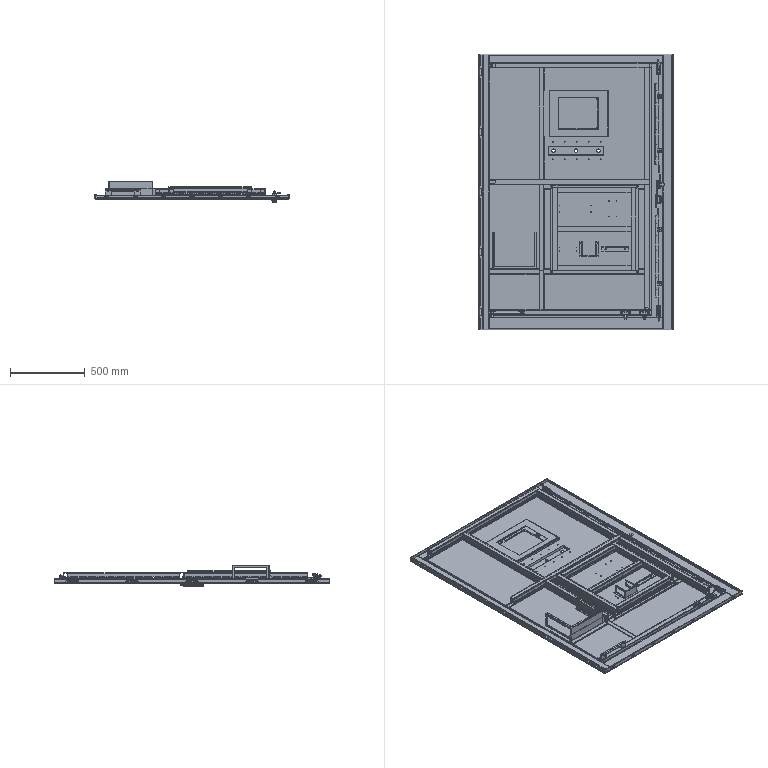Part | SolidWorks | 96 solids | 10969 faces | volume 12633746 mm3 | plane 6106 | cylinder 4045 | spline 639 | cone 144 | torus 30 | sphere 5 | commonest cylinder face diameters 8 x2044 1 x335 6 x153 2 x137 4 x126 3 x122